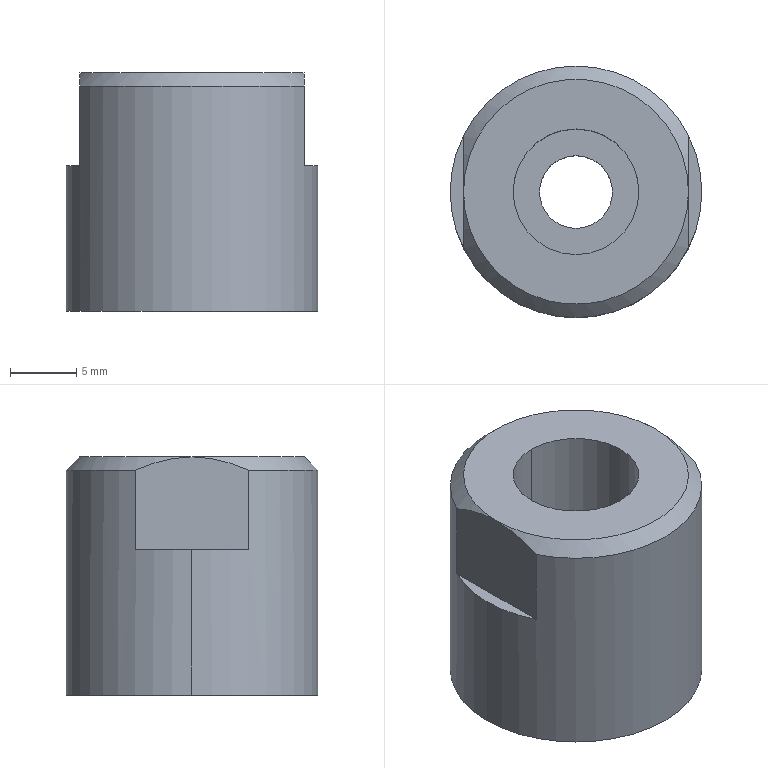Part | STEP file | J454-EBZ05-17-00-Part-1-16 | 1 solid | 15 faces | box 19 x 19 x 18 mm | volume 4103 mm3 | plane 7 | cylinder 6 | cone 2 | commonest cylinder face diameters 5.5 x2 9.5 x2 19 x2
STEP:
#1=CARTESIAN_POINT('',(0.,0.,0.));
#2=DIRECTION('',(0.,0.,1.));
#3=DIRECTION('',(1.,0.,0.));
#4=AXIS2_PLACEMENT_3D('',#1,#2,#3);
#5=CARTESIAN_POINT('',(0.,2.75,0.));
#6=VERTEX_POINT('',#5);
#7=CARTESIAN_POINT('',(0.,2.75,8.));
#8=VERTEX_POINT('',#7);
#9=CARTESIAN_POINT('',(0.,2.75,18.));
#10=DIRECTION('',(0.,0.,1.));
#11=VECTOR('',#10,1.);
#12=LINE('',#9,#11);
#13=CARTESIAN_POINT('',(0.,0.,18.));
#14=DIRECTION('',(0.,0.,1.));
#15=DIRECTION('',(0.,1.,0.));
#16=AXIS2_PLACEMENT_3D('',#13,#14,#15);
#17=CYLINDRICAL_SURFACE('',#16,2.75);
#18=CARTESIAN_POINT('',(6.283,0.));
#19=DIRECTION('',(0.,1.));
#20=VECTOR('',#19,1.);
#21=LINE('',#18,#20);
#22=(GEOMETRIC_REPRESENTATION_CONTEXT(2)PARAMETRIC_REPRESENTATION_CONTEXT()REPRESENTATION_CONTEXT('',''));
#23=DEFINITIONAL_REPRESENTATION('',(#21),#22);
#24=PCURVE('',#17,#23);
#25=CARTESIAN_POINT('',(0.,0.,18.));
#26=DIRECTION('',(0.,0.,1.));
#27=DIRECTION('',(0.,1.,0.));
#28=AXIS2_PLACEMENT_3D('',#25,#26,#27);
#29=CYLINDRICAL_SURFACE('',#28,2.75);
#30=CARTESIAN_POINT('',(0.,0.));
#31=DIRECTION('',(0.,1.));
#32=VECTOR('',#31,1.);
#33=LINE('',#30,#32);
#34=(GEOMETRIC_REPRESENTATION_CONTEXT(2)PARAMETRIC_REPRESENTATION_CONTEXT()REPRESENTATION_CONTEXT('',''));
#35=DEFINITIONAL_REPRESENTATION('',(#33),#34);
#36=PCURVE('',#29,#35);
#37=SURFACE_CURVE('',#12,(#24,#36),.PCURVE_S1.);
#38=EDGE_CURVE('',#6,#8,#37,.T.);
#39=ORIENTED_EDGE('',*,*,#38,.T.);
#40=CARTESIAN_POINT('',(0.,-2.75,8.));
#41=VERTEX_POINT('',#40);
#42=CARTESIAN_POINT('',(0.,0.,8.));
#43=DIRECTION('',(0.,0.,1.));
#44=DIRECTION('',(0.,1.,0.));
#45=AXIS2_PLACEMENT_3D('',#42,#43,#44);
#46=CIRCLE('',#45,2.75);
#47=CARTESIAN_POINT('',(0.,-10.));
#48=DIRECTION('',(1.,0.));
#49=VECTOR('',#48,1.);
#50=LINE('',#47,#49);
#51=(GEOMETRIC_REPRESENTATION_CONTEXT(2)PARAMETRIC_REPRESENTATION_CONTEXT()REPRESENTATION_CONTEXT('',''));
#52=DEFINITIONAL_REPRESENTATION('',(#50),#51);
#53=PCURVE('',#17,#52);
#54=CARTESIAN_POINT('',(0.,-4.75,8.));
#55=DIRECTION('',(0.,0.,-1.));
#56=DIRECTION('',(0.,-1.,0.));
#57=AXIS2_PLACEMENT_3D('',#54,#55,#56);
#58=PLANE('',#57);
#59=CARTESIAN_POINT('',(-7.5,0.));
#60=CARTESIAN_POINT('',(-7.5,4.763));
#61=CARTESIAN_POINT('',(-3.375,2.382));
#62=CARTESIAN_POINT('',(0.75,0.));
#63=CARTESIAN_POINT('',(-3.375,-2.382));
#64=CARTESIAN_POINT('',(-7.5,-4.763));
#65=CARTESIAN_POINT('',(-7.5,0.));
#66=(BOUNDED_CURVE()B_SPLINE_CURVE(2,(#59,#60,#61,#62,#63,#64,#65),.UNSPECIFIED.,.T.,.F.)B_SPLINE_CURVE_WITH_KNOTS((1,2,2,2,2,1),(-2.094,0.,2.094,4.189,6.283,8.378),.UNSPECIFIED.)CURVE()GEOMETRIC_REPRESENTATION_ITEM()RATIONAL_B_SPLINE_CURVE((1.,0.5,1.,0.5,1.,0.5,1.))REPRESENTATION_ITEM(''));
#67=(GEOMETRIC_REPRESENTATION_CONTEXT(2)PARAMETRIC_REPRESENTATION_CONTEXT()REPRESENTATION_CONTEXT('',''));
#68=DEFINITIONAL_REPRESENTATION('',(#66),#67);
#69=PCURVE('',#58,#68);
#70=SURFACE_CURVE('',#46,(#53,#69),.PCURVE_S1.);
#71=EDGE_CURVE('',#41,#8,#70,.T.);
#72=ORIENTED_EDGE('',*,*,#71,.F.);
#73=CARTESIAN_POINT('',(0.,-2.75,0.));
#74=VERTEX_POINT('',#73);
#75=CARTESIAN_POINT('',(0.,-2.75,18.));
#76=DIRECTION('',(0.,0.,1.));
#77=VECTOR('',#76,1.);
#78=LINE('',#75,#77);
#79=CARTESIAN_POINT('',(3.142,0.));
#80=DIRECTION('',(0.,1.));
#81=VECTOR('',#80,1.);
#82=LINE('',#79,#81);
#83=(GEOMETRIC_REPRESENTATION_CONTEXT(2)PARAMETRIC_REPRESENTATION_CONTEXT()REPRESENTATION_CONTEXT('',''));
#84=DEFINITIONAL_REPRESENTATION('',(#82),#83);
#85=PCURVE('',#17,#84);
#86=CARTESIAN_POINT('',(3.142,0.));
#87=DIRECTION('',(0.,1.));
#88=VECTOR('',#87,1.);
#89=LINE('',#86,#88);
#90=(GEOMETRIC_REPRESENTATION_CONTEXT(2)PARAMETRIC_REPRESENTATION_CONTEXT()REPRESENTATION_CONTEXT('',''));
#91=DEFINITIONAL_REPRESENTATION('',(#89),#90);
#92=PCURVE('',#29,#91);
#93=SURFACE_CURVE('',#78,(#85,#92),.PCURVE_S1.);
#94=EDGE_CURVE('',#74,#41,#93,.T.);
#95=ORIENTED_EDGE('',*,*,#94,.F.);
#96=CARTESIAN_POINT('',(0.,0.,0.));
#97=DIRECTION('',(0.,0.,1.));
#98=DIRECTION('',(0.,1.,0.));
#99=AXIS2_PLACEMENT_3D('',#96,#97,#98);
#100=CIRCLE('',#99,2.75);
#101=CARTESIAN_POINT('',(0.,-18.));
#102=DIRECTION('',(1.,0.));
#103=VECTOR('',#102,1.);
#104=LINE('',#101,#103);
#105=(GEOMETRIC_REPRESENTATION_CONTEXT(2)PARAMETRIC_REPRESENTATION_CONTEXT()REPRESENTATION_CONTEXT('',''));
#106=DEFINITIONAL_REPRESENTATION('',(#104),#105);
#107=PCURVE('',#17,#106);
#108=CARTESIAN_POINT('',(0.,0.,0.));
#109=DIRECTION('',(0.,0.,-1.));
#110=DIRECTION('',(-1.,0.,0.));
#111=AXIS2_PLACEMENT_3D('',#108,#109,#110);
#112=PLANE('',#111);
#113=CARTESIAN_POINT('',(0.,2.75));
#114=CARTESIAN_POINT('',(4.763,2.75));
#115=CARTESIAN_POINT('',(2.382,-1.375));
#116=CARTESIAN_POINT('',(0.,-5.5));
#117=CARTESIAN_POINT('',(-2.382,-1.375));
#118=CARTESIAN_POINT('',(-4.763,2.75));
#119=CARTESIAN_POINT('',(0.,2.75));
#120=(BOUNDED_CURVE()B_SPLINE_CURVE(2,(#113,#114,#115,#116,#117,#118,#119),.UNSPECIFIED.,.T.,.F.)B_SPLINE_CURVE_WITH_KNOTS((1,2,2,2,2,1),(-2.094,0.,2.094,4.189,6.283,8.378),.UNSPECIFIED.)CURVE()GEOMETRIC_REPRESENTATION_ITEM()RATIONAL_B_SPLINE_CURVE((1.,0.5,1.,0.5,1.,0.5,1.))REPRESENTATION_ITEM(''));
#121=(GEOMETRIC_REPRESENTATION_CONTEXT(2)PARAMETRIC_REPRESENTATION_CONTEXT()REPRESENTATION_CONTEXT('',''));
#122=DEFINITIONAL_REPRESENTATION('',(#120),#121);
#123=PCURVE('',#112,#122);
#124=SURFACE_CURVE('',#100,(#107,#123),.PCURVE_S1.);
#125=EDGE_CURVE('',#74,#6,#124,.T.);
#126=ORIENTED_EDGE('',*,*,#125,.T.);
#127=EDGE_LOOP('',(#39,#72,#95,#126));
#128=FACE_BOUND('',#127,.F.);
#129=ADVANCED_FACE('',(#128),#17,.F.);
#130=CARTESIAN_POINT('',(0.,4.75,8.));
#131=VERTEX_POINT('',#130);
#132=CARTESIAN_POINT('',(0.,4.75,18.));
#133=VERTEX_POINT('',#132);
#134=CARTESIAN_POINT('',(0.,4.75,18.));
#135=DIRECTION('',(0.,0.,1.));
#136=VECTOR('',#135,1.);
#137=LINE('',#134,#136);
#138=CARTESIAN_POINT('',(0.,0.,18.));
#139=DIRECTION('',(0.,0.,1.));
#140=DIRECTION('',(0.,1.,0.));
#141=AXIS2_PLACEMENT_3D('',#138,#139,#140);
#142=CYLINDRICAL_SURFACE('',#141,4.75);
#143=CARTESIAN_POINT('',(6.283,0.));
#144=DIRECTION('',(0.,1.));
#145=VECTOR('',#144,1.);
#146=LINE('',#143,#145);
#147=(GEOMETRIC_REPRESENTATION_CONTEXT(2)PARAMETRIC_REPRESENTATION_CONTEXT()REPRESENTATION_CONTEXT('',''));
#148=DEFINITIONAL_REPRESENTATION('',(#146),#147);
#149=PCURVE('',#142,#148);
#150=CARTESIAN_POINT('',(0.,0.,18.));
#151=DIRECTION('',(0.,0.,1.));
#152=DIRECTION('',(0.,1.,0.));
#153=AXIS2_PLACEMENT_3D('',#150,#151,#152);
#154=CYLINDRICAL_SURFACE('',#153,4.75);
#155=CARTESIAN_POINT('',(0.,0.));
#156=DIRECTION('',(0.,1.));
#157=VECTOR('',#156,1.);
#158=LINE('',#155,#157);
#159=(GEOMETRIC_REPRESENTATION_CONTEXT(2)PARAMETRIC_REPRESENTATION_CONTEXT()REPRESENTATION_CONTEXT('',''));
#160=DEFINITIONAL_REPRESENTATION('',(#158),#159);
#161=PCURVE('',#154,#160);
#162=SURFACE_CURVE('',#137,(#149,#161),.PCURVE_S1.);
#163=EDGE_CURVE('',#131,#133,#162,.T.);
#164=ORIENTED_EDGE('',*,*,#163,.T.);
#165=CARTESIAN_POINT('',(0.,-4.75,18.));
#166=VERTEX_POINT('',#165);
#167=CARTESIAN_POINT('',(0.,0.,18.));
#168=DIRECTION('',(0.,0.,1.));
#169=DIRECTION('',(0.,1.,0.));
#170=AXIS2_PLACEMENT_3D('',#167,#168,#169);
#171=CIRCLE('',#170,4.75);
#172=CARTESIAN_POINT('',(0.,0.));
#173=DIRECTION('',(1.,0.));
#174=VECTOR('',#173,1.);
#175=LINE('',#172,#174);
#176=(GEOMETRIC_REPRESENTATION_CONTEXT(2)PARAMETRIC_REPRESENTATION_CONTEXT()REPRESENTATION_CONTEXT('',''));
#177=DEFINITIONAL_REPRESENTATION('',(#175),#176);
#178=PCURVE('',#142,#177);
#179=CARTESIAN_POINT('',(0.,0.,18.));
#180=DIRECTION('',(0.,0.,1.));
#181=DIRECTION('',(1.,0.,0.));
#182=AXIS2_PLACEMENT_3D('',#179,#180,#181);
#183=PLANE('',#182);
#184=CARTESIAN_POINT('',(0.,0.));
#185=DIRECTION('',(0.,1.));
#186=AXIS2_PLACEMENT_2D('',#184,#185);
#187=CIRCLE('',#186,4.75);
#188=(GEOMETRIC_REPRESENTATION_CONTEXT(2)PARAMETRIC_REPRESENTATION_CONTEXT()REPRESENTATION_CONTEXT('',''));
#189=DEFINITIONAL_REPRESENTATION('',(#187),#188);
#190=PCURVE('',#183,#189);
#191=SURFACE_CURVE('',#171,(#178,#190),.PCURVE_S1.);
#192=EDGE_CURVE('',#166,#133,#191,.T.);
#193=ORIENTED_EDGE('',*,*,#192,.F.);
#194=CARTESIAN_POINT('',(0.,-4.75,8.));
#195=VERTEX_POINT('',#194);
#196=CARTESIAN_POINT('',(0.,-4.75,18.));
#197=DIRECTION('',(0.,0.,1.));
#198=VECTOR('',#197,1.);
#199=LINE('',#196,#198);
#200=CARTESIAN_POINT('',(3.142,0.));
#201=DIRECTION('',(0.,1.));
#202=VECTOR('',#201,1.);
#203=LINE('',#200,#202);
#204=(GEOMETRIC_REPRESENTATION_CONTEXT(2)PARAMETRIC_REPRESENTATION_CONTEXT()REPRESENTATION_CONTEXT('',''));
#205=DEFINITIONAL_REPRESENTATION('',(#203),#204);
#206=PCURVE('',#142,#205);
#207=CARTESIAN_POINT('',(3.142,0.));
#208=DIRECTION('',(0.,1.));
#209=VECTOR('',#208,1.);
#210=LINE('',#207,#209);
#211=(GEOMETRIC_REPRESENTATION_CONTEXT(2)PARAMETRIC_REPRESENTATION_CONTEXT()REPRESENTATION_CONTEXT('',''));
#212=DEFINITIONAL_REPRESENTATION('',(#210),#211);
#213=PCURVE('',#154,#212);
#214=SURFACE_CURVE('',#199,(#206,#213),.PCURVE_S1.);
#215=EDGE_CURVE('',#195,#166,#214,.T.);
#216=ORIENTED_EDGE('',*,*,#215,.F.);
#217=CARTESIAN_POINT('',(0.,0.,8.));
#218=DIRECTION('',(0.,0.,1.));
#219=DIRECTION('',(0.,1.,0.));
#220=AXIS2_PLACEMENT_3D('',#217,#218,#219);
#221=CIRCLE('',#220,4.75);
#222=CARTESIAN_POINT('',(0.,-10.));
#223=DIRECTION('',(1.,0.));
#224=VECTOR('',#223,1.);
#225=LINE('',#222,#224);
#226=(GEOMETRIC_REPRESENTATION_CONTEXT(2)PARAMETRIC_REPRESENTATION_CONTEXT()REPRESENTATION_CONTEXT('',''));
#227=DEFINITIONAL_REPRESENTATION('',(#225),#226);
#228=PCURVE('',#142,#227);
#229=CARTESIAN_POINT('',(-9.5,0.));
#230=CARTESIAN_POINT('',(-9.5,8.227));
#231=CARTESIAN_POINT('',(-2.375,4.114));
#232=CARTESIAN_POINT('',(4.75,0.));
#233=CARTESIAN_POINT('',(-2.375,-4.114));
#234=CARTESIAN_POINT('',(-9.5,-8.227));
#235=CARTESIAN_POINT('',(-9.5,0.));
#236=(BOUNDED_CURVE()B_SPLINE_CURVE(2,(#229,#230,#231,#232,#233,#234,#235),.UNSPECIFIED.,.T.,.F.)B_SPLINE_CURVE_WITH_KNOTS((1,2,2,2,2,1),(-2.094,0.,2.094,4.189,6.283,8.378),.UNSPECIFIED.)CURVE()GEOMETRIC_REPRESENTATION_ITEM()RATIONAL_B_SPLINE_CURVE((1.,0.5,1.,0.5,1.,0.5,1.))REPRESENTATION_ITEM(''));
#237=(GEOMETRIC_REPRESENTATION_CONTEXT(2)PARAMETRIC_REPRESENTATION_CONTEXT()REPRESENTATION_CONTEXT('',''));
#238=DEFINITIONAL_REPRESENTATION('',(#236),#237);
#239=PCURVE('',#58,#238);
#240=SURFACE_CURVE('',#221,(#228,#239),.PCURVE_S1.);
#241=EDGE_CURVE('',#195,#131,#240,.T.);
#242=ORIENTED_EDGE('',*,*,#241,.T.);
#243=EDGE_LOOP('',(#164,#193,#216,#242));
#244=FACE_BOUND('',#243,.F.);
#245=ADVANCED_FACE('',(#244),#142,.F.);
#246=CARTESIAN_POINT('',(9.5,0.,0.));
#247=VERTEX_POINT('',#246);
#248=CARTESIAN_POINT('',(-9.5,0.,0.));
#249=VERTEX_POINT('',#248);
#250=CARTESIAN_POINT('',(0.,0.,0.));
#251=DIRECTION('',(0.,0.,1.));
#252=DIRECTION('',(1.,0.,0.));
#253=AXIS2_PLACEMENT_3D('',#250,#251,#252);
#254=CIRCLE('',#253,9.5);
#255=CARTESIAN_POINT('',(0.,0.,0.));
#256=DIRECTION('',(0.,0.,1.));
#257=DIRECTION('',(1.,0.,0.));
#258=AXIS2_PLACEMENT_3D('',#255,#256,#257);
#259=CYLINDRICAL_SURFACE('',#258,9.5);
#260=CARTESIAN_POINT('',(0.,0.));
#261=DIRECTION('',(1.,0.));
#262=VECTOR('',#261,1.);
#263=LINE('',#260,#262);
#264=(GEOMETRIC_REPRESENTATION_CONTEXT(2)PARAMETRIC_REPRESENTATION_CONTEXT()REPRESENTATION_CONTEXT('',''));
#265=DEFINITIONAL_REPRESENTATION('',(#263),#264);
#266=PCURVE('',#259,#265);
#267=CARTESIAN_POINT('',(-9.5,0.));
#268=CARTESIAN_POINT('',(-9.5,16.454));
#269=CARTESIAN_POINT('',(4.75,8.227));
#270=CARTESIAN_POINT('',(19.,0.));
#271=CARTESIAN_POINT('',(4.75,-8.227));
#272=CARTESIAN_POINT('',(-9.5,-16.454));
#273=CARTESIAN_POINT('',(-9.5,0.));
#274=(BOUNDED_CURVE()B_SPLINE_CURVE(2,(#267,#268,#269,#270,#271,#272,#273),.UNSPECIFIED.,.T.,.F.)B_SPLINE_CURVE_WITH_KNOTS((1,2,2,2,2,1),(-2.094,0.,2.094,4.189,6.283,8.378),.UNSPECIFIED.)CURVE()GEOMETRIC_REPRESENTATION_ITEM()RATIONAL_B_SPLINE_CURVE((1.,0.5,1.,0.5,1.,0.5,1.))REPRESENTATION_ITEM(''));
#275=(GEOMETRIC_REPRESENTATION_CONTEXT(2)PARAMETRIC_REPRESENTATION_CONTEXT()REPRESENTATION_CONTEXT('',''));
#276=DEFINITIONAL_REPRESENTATION('',(#274),#275);
#277=PCURVE('',#112,#276);
#278=SURFACE_CURVE('',#254,(#266,#277),.PCURVE_S1.);
#279=EDGE_CURVE('',#247,#249,#278,.T.);
#280=ORIENTED_EDGE('',*,*,#279,.T.);
#281=CARTESIAN_POINT('',(-9.5,0.,11.));
#282=VERTEX_POINT('',#281);
#283=CARTESIAN_POINT('',(-9.5,0.,0.));
#284=DIRECTION('',(0.,0.,1.));
#285=VECTOR('',#284,1.);
#286=LINE('',#283,#285);
#287=CARTESIAN_POINT('',(3.142,0.));
#288=DIRECTION('',(0.,1.));
#289=VECTOR('',#288,1.);
#290=LINE('',#287,#289);
#291=(GEOMETRIC_REPRESENTATION_CONTEXT(2)PARAMETRIC_REPRESENTATION_CONTEXT()REPRESENTATION_CONTEXT('',''));
#292=DEFINITIONAL_REPRESENTATION('',(#290),#291);
#293=PCURVE('',#259,#292);
#294=CARTESIAN_POINT('',(0.,0.,0.));
#295=DIRECTION('',(0.,0.,1.));
#296=DIRECTION('',(1.,0.,0.));
#297=AXIS2_PLACEMENT_3D('',#294,#295,#296);
#298=CYLINDRICAL_SURFACE('',#297,9.5);
#299=CARTESIAN_POINT('',(3.142,0.));
#300=DIRECTION('',(0.,1.));
#301=VECTOR('',#300,1.);
#302=LINE('',#299,#301);
#303=(GEOMETRIC_REPRESENTATION_CONTEXT(2)PARAMETRIC_REPRESENTATION_CONTEXT()REPRESENTATION_CONTEXT('',''));
#304=DEFINITIONAL_REPRESENTATION('',(#302),#303);
#305=PCURVE('',#298,#304);
#306=SURFACE_CURVE('',#286,(#293,#305),.PCURVE_S1.);
#307=EDGE_CURVE('',#249,#282,#306,.T.);
#308=ORIENTED_EDGE('',*,*,#307,.T.);
#309=CARTESIAN_POINT('',(-8.5,4.243,11.));
#310=VERTEX_POINT('',#309);
#311=CARTESIAN_POINT('',(0.,0.,11.));
#312=DIRECTION('',(0.,0.,1.));
#313=DIRECTION('',(-1.,0.,0.));
#314=AXIS2_PLACEMENT_3D('',#311,#312,#313);
#315=CIRCLE('',#314,9.5);
#316=CARTESIAN_POINT('',(-3.142,11.));
#317=DIRECTION('',(1.,0.));
#318=VECTOR('',#317,1.);
#319=LINE('',#316,#318);
#320=(GEOMETRIC_REPRESENTATION_CONTEXT(2)PARAMETRIC_REPRESENTATION_CONTEXT()REPRESENTATION_CONTEXT('',''));
#321=DEFINITIONAL_REPRESENTATION('',(#319),#320);
#322=PCURVE('',#259,#321);
#323=CARTESIAN_POINT('',(-19.25,-7.5,11.));
#324=DIRECTION('',(0.,0.,-1.));
#325=DIRECTION('',(0.,-1.,0.));
#326=AXIS2_PLACEMENT_3D('',#323,#324,#325);
#327=PLANE('',#326);
#328=CARTESIAN_POINT('',(-7.5,-9.75));
#329=CARTESIAN_POINT('',(8.954,-9.75));
#330=CARTESIAN_POINT('',(0.7272,-24.));
#331=CARTESIAN_POINT('',(-7.5,-38.25));
#332=CARTESIAN_POINT('',(-15.727,-24.));
#333=CARTESIAN_POINT('',(-23.954,-9.75));
#334=CARTESIAN_POINT('',(-7.5,-9.75));
#335=(BOUNDED_CURVE()B_SPLINE_CURVE(2,(#328,#329,#330,#331,#332,#333,#334),.UNSPECIFIED.,.T.,.F.)B_SPLINE_CURVE_WITH_KNOTS((1,2,2,2,2,1),(-2.094,0.,2.094,4.189,6.283,8.378),.UNSPECIFIED.)CURVE()GEOMETRIC_REPRESENTATION_ITEM()RATIONAL_B_SPLINE_CURVE((1.,0.5,1.,0.5,1.,0.5,1.))REPRESENTATION_ITEM(''));
#336=(GEOMETRIC_REPRESENTATION_CONTEXT(2)PARAMETRIC_REPRESENTATION_CONTEXT()REPRESENTATION_CONTEXT('',''));
#337=DEFINITIONAL_REPRESENTATION('',(#335),#336);
#338=PCURVE('',#327,#337);
#339=SURFACE_CURVE('',#315,(#322,#338),.PCURVE_S1.);
#340=EDGE_CURVE('',#310,#282,#339,.T.);
#341=ORIENTED_EDGE('',*,*,#340,.F.);
#342=CARTESIAN_POINT('',(-8.5,4.243,17.));
#343=VERTEX_POINT('',#342);
#344=CARTESIAN_POINT('',(-8.5,4.243,0.));
#345=DIRECTION('',(0.,0.,-1.));
#346=VECTOR('',#345,1.);
#347=LINE('',#344,#346);
#348=CARTESIAN_POINT('',(2.679,0.));
#349=DIRECTION('',(0.,-1.));
#350=VECTOR('',#349,1.);
#351=LINE('',#348,#350);
#352=(GEOMETRIC_REPRESENTATION_CONTEXT(2)PARAMETRIC_REPRESENTATION_CONTEXT()REPRESENTATION_CONTEXT('',''));
#353=DEFINITIONAL_REPRESENTATION('',(#351),#352);
#354=PCURVE('',#259,#353);
#355=CARTESIAN_POINT('',(-8.5,-7.5,14.5));
#356=DIRECTION('',(1.,0.,0.));
#357=DIRECTION('',(0.,1.,0.));
#358=AXIS2_PLACEMENT_3D('',#355,#356,#357);
#359=PLANE('',#358);
#360=CARTESIAN_POINT('',(11.743,-14.5));
#361=DIRECTION('',(0.,-1.));
#362=VECTOR('',#361,1.);
#363=LINE('',#360,#362);
#364=(GEOMETRIC_REPRESENTATION_CONTEXT(2)PARAMETRIC_REPRESENTATION_CONTEXT()REPRESENTATION_CONTEXT('',''));
#365=DEFINITIONAL_REPRESENTATION('',(#363),#364);
#366=PCURVE('',#359,#365);
#367=SURFACE_CURVE('',#347,(#354,#366),.PCURVE_S1.);
#368=EDGE_CURVE('',#343,#310,#367,.T.);
#369=ORIENTED_EDGE('',*,*,#368,.F.);
#370=CARTESIAN_POINT('',(8.5,4.243,17.));
#371=VERTEX_POINT('',#370);
#372=CARTESIAN_POINT('',(0.,0.,17.));
#373=DIRECTION('',(0.,0.,-1.));
#374=DIRECTION('',(1.,0.,0.));
#375=AXIS2_PLACEMENT_3D('',#372,#373,#374);
#376=CIRCLE('',#375,9.5);
#377=CARTESIAN_POINT('',(6.283,17.));
#378=DIRECTION('',(-1.,0.));
#379=VECTOR('',#378,1.);
#380=LINE('',#377,#379);
#381=(GEOMETRIC_REPRESENTATION_CONTEXT(2)PARAMETRIC_REPRESENTATION_CONTEXT()REPRESENTATION_CONTEXT('',''));
#382=DEFINITIONAL_REPRESENTATION('',(#380),#381);
#383=PCURVE('',#259,#382);
#384=CARTESIAN_POINT('',(0.,0.,17.));
#385=DIRECTION('',(0.,0.,-1.));
#386=DIRECTION('',(-1.,0.,0.));
#387=AXIS2_PLACEMENT_3D('',#384,#385,#386);
#388=CONICAL_SURFACE('',#387,9.5,0.7854);
#389=CARTESIAN_POINT('',(-3.142,0.));
#390=DIRECTION('',(1.,0.));
#391=VECTOR('',#390,1.);
#392=LINE('',#389,#391);
#393=(GEOMETRIC_REPRESENTATION_CONTEXT(2)PARAMETRIC_REPRESENTATION_CONTEXT()REPRESENTATION_CONTEXT('',''));
#394=DEFINITIONAL_REPRESENTATION('',(#392),#393);
#395=PCURVE('',#388,#394);
#396=SURFACE_CURVE('',#376,(#383,#395),.PCURVE_S1.);
#397=EDGE_CURVE('',#343,#371,#396,.T.);
#398=ORIENTED_EDGE('',*,*,#397,.T.);
#399=CARTESIAN_POINT('',(8.5,4.243,11.));
#400=VERTEX_POINT('',#399);
#401=CARTESIAN_POINT('',(8.5,4.243,0.));
#402=DIRECTION('',(0.,0.,1.));
#403=VECTOR('',#402,1.);
#404=LINE('',#401,#403);
#405=CARTESIAN_POINT('',(0.463,0.));
#406=DIRECTION('',(0.,1.));
#407=VECTOR('',#406,1.);
#408=LINE('',#405,#407);
#409=(GEOMETRIC_REPRESENTATION_CONTEXT(2)PARAMETRIC_REPRESENTATION_CONTEXT()REPRESENTATION_CONTEXT('',''));
#410=DEFINITIONAL_REPRESENTATION('',(#408),#409);
#411=PCURVE('',#259,#410);
#412=CARTESIAN_POINT('',(8.5,7.5,14.5));
#413=DIRECTION('',(-1.,0.,0.));
#414=DIRECTION('',(0.,-1.,0.));
#415=AXIS2_PLACEMENT_3D('',#412,#413,#414);
#416=PLANE('',#415);
#417=CARTESIAN_POINT('',(3.257,-14.5));
#418=DIRECTION('',(0.,1.));
#419=VECTOR('',#418,1.);
#420=LINE('',#417,#419);
#421=(GEOMETRIC_REPRESENTATION_CONTEXT(2)PARAMETRIC_REPRESENTATION_CONTEXT()REPRESENTATION_CONTEXT('',''));
#422=DEFINITIONAL_REPRESENTATION('',(#420),#421);
#423=PCURVE('',#416,#422);
#424=SURFACE_CURVE('',#404,(#411,#423),.PCURVE_S1.);
#425=EDGE_CURVE('',#400,#371,#424,.T.);
#426=ORIENTED_EDGE('',*,*,#425,.F.);
#427=CARTESIAN_POINT('',(9.5,0.,11.));
#428=VERTEX_POINT('',#427);
#429=CARTESIAN_POINT('',(0.,0.,11.));
#430=DIRECTION('',(0.,0.,1.));
#431=DIRECTION('',(-1.,0.,0.));
#432=AXIS2_PLACEMENT_3D('',#429,#430,#431);
#433=CIRCLE('',#432,9.5);
#434=CARTESIAN_POINT('',(-3.142,11.));
#435=DIRECTION('',(1.,0.));
#436=VECTOR('',#435,1.);
#437=LINE('',#434,#436);
#438=(GEOMETRIC_REPRESENTATION_CONTEXT(2)PARAMETRIC_REPRESENTATION_CONTEXT()REPRESENTATION_CONTEXT('',''));
#439=DEFINITIONAL_REPRESENTATION('',(#437),#438);
#440=PCURVE('',#259,#439);
#441=CARTESIAN_POINT('',(19.25,7.5,11.));
#442=DIRECTION('',(0.,0.,-1.));
#443=DIRECTION('',(0.,1.,0.));
#444=AXIS2_PLACEMENT_3D('',#441,#442,#443);
#445=PLANE('',#444);
#446=CARTESIAN_POINT('',(-7.5,-28.75));
#447=CARTESIAN_POINT('',(-23.954,-28.75));
#448=CARTESIAN_POINT('',(-15.727,-14.5));
#449=CARTESIAN_POINT('',(-7.5,-0.25));
#450=CARTESIAN_POINT('',(0.7272,-14.5));
#451=CARTESIAN_POINT('',(8.954,-28.75));
#452=CARTESIAN_POINT('',(-7.5,-28.75));
#453=(BOUNDED_CURVE()B_SPLINE_CURVE(2,(#446,#447,#448,#449,#450,#451,#452),.UNSPECIFIED.,.T.,.F.)B_SPLINE_CURVE_WITH_KNOTS((1,2,2,2,2,1),(-2.094,0.,2.094,4.189,6.283,8.378),.UNSPECIFIED.)CURVE()GEOMETRIC_REPRESENTATION_ITEM()RATIONAL_B_SPLINE_CURVE((1.,0.5,1.,0.5,1.,0.5,1.))REPRESENTATION_ITEM(''));
#454=(GEOMETRIC_REPRESENTATION_CONTEXT(2)PARAMETRIC_REPRESENTATION_CONTEXT()REPRESENTATION_CONTEXT('',''));
#455=DEFINITIONAL_REPRESENTATION('',(#453),#454);
#456=PCURVE('',#445,#455);
#457=SURFACE_CURVE('',#433,(#440,#456),.PCURVE_S1.);
#458=EDGE_CURVE('',#428,#400,#457,.T.);
#459=ORIENTED_EDGE('',*,*,#458,.F.);
#460=CARTESIAN_POINT('',(9.5,0.,0.));
#461=DIRECTION('',(0.,0.,1.));
#462=VECTOR('',#461,1.);
#463=LINE('',#460,#462);
#464=CARTESIAN_POINT('',(0.,0.));
#465=DIRECTION('',(0.,1.));
#466=VECTOR('',#465,1.);
#467=LINE('',#464,#466);
#468=(GEOMETRIC_REPRESENTATION_CONTEXT(2)PARAMETRIC_REPRESENTATION_CONTEXT()REPRESENTATION_CONTEXT('',''));
#469=DEFINITIONAL_REPRESENTATION('',(#467),#468);
#470=PCURVE('',#259,#469);
#471=CARTESIAN_POINT('',(6.283,0.));
#472=DIRECTION('',(0.,1.));
#473=VECTOR('',#472,1.);
#474=LINE('',#471,#473);
#475=(GEOMETRIC_REPRESENTATION_CONTEXT(2)PARAMETRIC_REPRESENTATION_CONTEXT()REPRESENTATION_CONTEXT('',''));
#476=DEFINITIONAL_REPRESENTATION('',(#474),#475);
#477=PCURVE('',#298,#476);
#478=SURFACE_CURVE('',#463,(#470,#477),.PCURVE_S1.);
#479=EDGE_CURVE('',#247,#428,#478,.T.);
#480=ORIENTED_EDGE('',*,*,#479,.F.);
#481=EDGE_LOOP('',(#280,#308,#341,#369,#398,#426,#459,#480));
#482=FACE_BOUND('',#481,.T.);
#483=ADVANCED_FACE('',(#482),#259,.T.);
#484=CARTESIAN_POINT('',(8.5,0.,18.));
#485=VERTEX_POINT('',#484);
#486=CARTESIAN_POINT('',(8.5,4.243,17.));
#487=CARTESIAN_POINT('',(8.5,3.909,17.149));
#488=CARTESIAN_POINT('',(8.5,3.57,17.287));
#489=CARTESIAN_POINT('',(8.5,2.877,17.532));
#490=CARTESIAN_POINT('',(8.5,2.524,17.64));
#491=CARTESIAN_POINT('',(8.5,1.459,17.903));
#492=CARTESIAN_POINT('',(8.5,0.737,18.));
#493=CARTESIAN_POINT('',(8.5,0.,18.));
#494=B_SPLINE_CURVE_WITH_KNOTS('',3,(#486,#487,#488,#489,#490,#491,#492,#493),.UNSPECIFIED.,.F.,.F.,(4,2,2,4),(0.02347,0.02457,0.02567,0.02786),.UNSPECIFIED.);
#495=CARTESIAN_POINT('',(2.679,0.));
#496=CARTESIAN_POINT('',(2.684,-0.0271));
#497=CARTESIAN_POINT('',(2.696,-0.08054));
#498=CARTESIAN_POINT('',(2.714,-0.1583));
#499=CARTESIAN_POINT('',(2.732,-0.2335));
#500=CARTESIAN_POINT('',(2.75,-0.3061));
#501=CARTESIAN_POINT('',(2.769,-0.376));
#502=CARTESIAN_POINT('',(2.789,-0.443));
#503=CARTESIAN_POINT('',(2.809,-0.5069));
#504=CARTESIAN_POINT('',(2.829,-0.5676));
#505=CARTESIAN_POINT('',(2.85,-0.6249));
#506=CARTESIAN_POINT('',(2.87,-0.6785));
#507=CARTESIAN_POINT('',(2.892,-0.7283));
#508=CARTESIAN_POINT('',(2.913,-0.7742));
#509=CARTESIAN_POINT('',(2.935,-0.8162));
#510=CARTESIAN_POINT('',(2.957,-0.8541));
#511=CARTESIAN_POINT('',(2.98,-0.8878));
#512=CARTESIAN_POINT('',(3.002,-0.9173));
#513=CARTESIAN_POINT('',(3.025,-0.9425));
#514=CARTESIAN_POINT('',(3.048,-0.9633));
#515=CARTESIAN_POINT('',(3.071,-0.9796));
#516=CARTESIAN_POINT('',(3.094,-0.9913));
#517=CARTESIAN_POINT('',(3.118,-0.9984));
#518=CARTESIAN_POINT('',(3.134,-1.));
#519=CARTESIAN_POINT('',(3.142,-1.));
#520=B_SPLINE_CURVE_WITH_KNOTS('',3,(#495,#496,#497,#498,#499,#500,#501,#502,#503,#504,#505,#506,#507,#508,#509,#510,#511,#512,#513,#514,#515,#516,#517,#518,#519),.UNSPECIFIED.,.F.,.F.,(4,1,1,1,1,1,1,1,1,1,1,1,1,1,1,1,1,1,1,1,1,1,4),(0.02347,0.02367,0.02387,0.02407,0.02427,0.02447,0.02467,0.02487,0.02507,0.02527,0.02547,0.02567,0.02587,0.02607,0.02627,0.02647,0.02667,0.02687,0.02707,0.02727,0.02747,0.02766,0.02786),.QUASI_UNIFORM_KNOTS.);
#521=(GEOMETRIC_REPRESENTATION_CONTEXT(2)PARAMETRIC_REPRESENTATION_CONTEXT()REPRESENTATION_CONTEXT('',''));
#522=DEFINITIONAL_REPRESENTATION('',(#520),#521);
#523=PCURVE('',#388,#522);
#524=CARTESIAN_POINT('',(3.257,2.5));
#525=CARTESIAN_POINT('',(3.591,2.649));
#526=CARTESIAN_POINT('',(3.93,2.787));
#527=CARTESIAN_POINT('',(4.623,3.032));
#528=CARTESIAN_POINT('',(4.976,3.14));
#529=CARTESIAN_POINT('',(6.041,3.403));
#530=CARTESIAN_POINT('',(6.763,3.5));
#531=CARTESIAN_POINT('',(7.5,3.5));
#532=B_SPLINE_CURVE_WITH_KNOTS('',3,(#524,#525,#526,#527,#528,#529,#530,#531),.UNSPECIFIED.,.F.,.F.,(4,2,2,4),(0.02347,0.02457,0.02567,0.02786),.UNSPECIFIED.);
#533=(GEOMETRIC_REPRESENTATION_CONTEXT(2)PARAMETRIC_REPRESENTATION_CONTEXT()REPRESENTATION_CONTEXT('',''));
#534=DEFINITIONAL_REPRESENTATION('',(#532),#533);
#535=PCURVE('',#416,#534);
#536=SURFACE_CURVE('',#494,(#523,#535),.PCURVE_S1.);
#537=EDGE_CURVE('',#371,#485,#536,.T.);
#538=ORIENTED_EDGE('',*,*,#537,.F.);
#539=ORIENTED_EDGE('',*,*,#397,.F.);
#540=CARTESIAN_POINT('',(-8.5,0.,18.));
#541=VERTEX_POINT('',#540);
#542=CARTESIAN_POINT('',(-8.5,0.,18.));
#543=CARTESIAN_POINT('',(-8.5,0.3684,18.));
#544=CARTESIAN_POINT('',(-8.5,0.7366,17.976));
#545=CARTESIAN_POINT('',(-8.5,1.461,17.883));
#546=CARTESIAN_POINT('',(-8.5,1.818,17.814));
#547=CARTESIAN_POINT('',(-8.5,2.881,17.551));
#548=CARTESIAN_POINT('',(-8.5,3.578,17.297));
#549=CARTESIAN_POINT('',(-8.5,4.243,17.));
#550=B_SPLINE_CURVE_WITH_KNOTS('',3,(#542,#543,#544,#545,#546,#547,#548,#549),.UNSPECIFIED.,.F.,.F.,(4,2,2,4),(0.02786,0.02896,0.03006,0.03225),.UNSPECIFIED.);
#551=CARTESIAN_POINT('',(0.,-1.));
#552=CARTESIAN_POINT('',(0.00788,-1.));
#553=CARTESIAN_POINT('',(0.02364,-0.9984));
#554=CARTESIAN_POINT('',(0.04722,-0.9913));
#555=CARTESIAN_POINT('',(0.0707,-0.9795));
#556=CARTESIAN_POINT('',(0.09401,-0.9631));
#557=CARTESIAN_POINT('',(0.1171,-0.9421));
#558=CARTESIAN_POINT('',(0.14,-0.9168));
#559=CARTESIAN_POINT('',(0.1626,-0.8872));
#560=CARTESIAN_POINT('',(0.1849,-0.8533));
#561=CARTESIAN_POINT('',(0.207,-0.8153));
#562=CARTESIAN_POINT('',(0.2288,-0.7733));
#563=CARTESIAN_POINT('',(0.2503,-0.7274));
#564=CARTESIAN_POINT('',(0.2715,-0.6776));
#565=CARTESIAN_POINT('',(0.2923,-0.6241));
#566=CARTESIAN_POINT('',(0.3129,-0.567));
#567=CARTESIAN_POINT('',(0.333,-0.5065));
#568=CARTESIAN_POINT('',(0.3528,-0.4427));
#569=CARTESIAN_POINT('',(0.3722,-0.3757));
#570=CARTESIAN_POINT('',(0.3912,-0.3059));
#571=CARTESIAN_POINT('',(0.4098,-0.2332));
#572=CARTESIAN_POINT('',(0.428,-0.158));
#573=CARTESIAN_POINT('',(0.4457,-0.08029));
#574=CARTESIAN_POINT('',(0.4573,-0.02699));
#575=CARTESIAN_POINT('',(0.463,0.));
#576=B_SPLINE_CURVE_WITH_KNOTS('',3,(#551,#552,#553,#554,#555,#556,#557,#558,#559,#560,#561,#562,#563,#564,#565,#566,#567,#568,#569,#570,#571,#572,#573,#574,#575),.UNSPECIFIED.,.F.,.F.,(4,1,1,1,1,1,1,1,1,1,1,1,1,1,1,1,1,1,1,1,1,1,4),(0.02786,0.02806,0.02826,0.02846,0.02866,0.02886,0.02906,0.02926,0.02946,0.02966,0.02986,0.03006,0.03026,0.03046,0.03066,0.03086,0.03106,0.03126,0.03145,0.03165,0.03185,0.03205,0.03225),.QUASI_UNIFORM_KNOTS.);
#577=(GEOMETRIC_REPRESENTATION_CONTEXT(2)PARAMETRIC_REPRESENTATION_CONTEXT()REPRESENTATION_CONTEXT('',''));
#578=DEFINITIONAL_REPRESENTATION('',(#576),#577);
#579=PCURVE('',#388,#578);
#580=CARTESIAN_POINT('',(7.5,3.5));
#581=CARTESIAN_POINT('',(7.868,3.5));
#582=CARTESIAN_POINT('',(8.237,3.476));
#583=CARTESIAN_POINT('',(8.961,3.383));
#584=CARTESIAN_POINT('',(9.318,3.314));
#585=CARTESIAN_POINT('',(10.381,3.051));
#586=CARTESIAN_POINT('',(11.078,2.797));
#587=CARTESIAN_POINT('',(11.743,2.5));
#588=B_SPLINE_CURVE_WITH_KNOTS('',3,(#580,#581,#582,#583,#584,#585,#586,#587),.UNSPECIFIED.,.F.,.F.,(4,2,2,4),(0.02786,0.02896,0.03006,0.03225),.UNSPECIFIED.);
#589=(GEOMETRIC_REPRESENTATION_CONTEXT(2)PARAMETRIC_REPRESENTATION_CONTEXT()REPRESENTATION_CONTEXT('',''));
#590=DEFINITIONAL_REPRESENTATION('',(#588),#589);
#591=PCURVE('',#359,#590);
#592=SURFACE_CURVE('',#550,(#579,#591),.PCURVE_S1.);
#593=EDGE_CURVE('',#541,#343,#592,.T.);
#594=ORIENTED_EDGE('',*,*,#593,.F.);
#595=CARTESIAN_POINT('',(0.,0.,18.));
#596=DIRECTION('',(0.,0.,1.));
#597=DIRECTION('',(1.,0.,0.));
#598=AXIS2_PLACEMENT_3D('',#595,#596,#597);
#599=CIRCLE('',#598,8.5);
#600=CARTESIAN_POINT('',(3.142,-1.));
#601=DIRECTION('',(-1.,0.));
#602=VECTOR('',#601,1.);
#603=LINE('',#600,#602);
#604=(GEOMETRIC_REPRESENTATION_CONTEXT(2)PARAMETRIC_REPRESENTATION_CONTEXT()REPRESENTATION_CONTEXT('',''));
#605=DEFINITIONAL_REPRESENTATION('',(#603),#604);
#606=PCURVE('',#388,#605);
#607=CARTESIAN_POINT('',(0.,0.));
#608=DIRECTION('',(1.,0.));
#609=AXIS2_PLACEMENT_2D('',#607,#608);
#610=CIRCLE('',#609,8.5);
#611=(GEOMETRIC_REPRESENTATION_CONTEXT(2)PARAMETRIC_REPRESENTATION_CONTEXT()REPRESENTATION_CONTEXT('',''));
#612=DEFINITIONAL_REPRESENTATION('',(#610),#611);
#613=PCURVE('',#183,#612);
#614=SURFACE_CURVE('',#599,(#606,#613),.PCURVE_S1.);
#615=EDGE_CURVE('',#485,#541,#614,.T.);
#616=ORIENTED_EDGE('',*,*,#615,.F.);
#617=EDGE_LOOP('',(#538,#539,#594,#616));
#618=FACE_BOUND('',#617,.T.);
#619=ADVANCED_FACE('',(#618),#388,.T.);
#620=CARTESIAN_POINT('',(0.,0.,18.));
#621=DIRECTION('',(0.,0.,1.));
#622=DIRECTION('',(0.,1.,0.));
#623=AXIS2_PLACEMENT_3D('',#620,#621,#622);
#624=CIRCLE('',#623,4.75);
#625=CARTESIAN_POINT('',(0.,0.));
#626=DIRECTION('',(0.,1.));
#627=AXIS2_PLACEMENT_2D('',#625,#626);
#628=CIRCLE('',#627,4.75);
#629=(GEOMETRIC_REPRESENTATION_CONTEXT(2)PARAMETRIC_REPRESENTATION_CONTEXT()REPRESENTATION_CONTEXT('',''));
#630=DEFINITIONAL_REPRESENTATION('',(#628),#629);
#631=PCURVE('',#183,#630);
#632=CARTESIAN_POINT('',(0.,0.));
#633=DIRECTION('',(1.,0.));
#634=VECTOR('',#633,1.);
#635=LINE('',#632,#634);
#636=(GEOMETRIC_REPRESENTATION_CONTEXT(2)PARAMETRIC_REPRESENTATION_CONTEXT()REPRESENTATION_CONTEXT('',''));
#637=DEFINITIONAL_REPRESENTATION('',(#635),#636);
#638=PCURVE('',#154,#637);
#639=SURFACE_CURVE('',#624,(#631,#638),.PCURVE_S1.);
#640=EDGE_CURVE('',#133,#166,#639,.T.);
#641=ORIENTED_EDGE('',*,*,#640,.F.);
#642=ORIENTED_EDGE('',*,*,#192,.F.);
#643=EDGE_LOOP('',(#641,#642));
#644=FACE_BOUND('',#643,.T.);
#645=CARTESIAN_POINT('',(0.,0.,18.));
#646=DIRECTION('',(0.,0.,1.));
#647=DIRECTION('',(1.,0.,0.));
#648=AXIS2_PLACEMENT_3D('',#645,#646,#647);
#649=CIRCLE('',#648,8.5);
#650=CARTESIAN_POINT('',(0.,0.));
#651=DIRECTION('',(1.,0.));
#652=AXIS2_PLACEMENT_2D('',#650,#651);
#653=CIRCLE('',#652,8.5);
#654=(GEOMETRIC_REPRESENTATION_CONTEXT(2)PARAMETRIC_REPRESENTATION_CONTEXT()REPRESENTATION_CONTEXT('',''));
#655=DEFINITIONAL_REPRESENTATION('',(#653),#654);
#656=PCURVE('',#183,#655);
#657=CARTESIAN_POINT('',(0.,0.,17.));
#658=DIRECTION('',(0.,0.,-1.));
#659=DIRECTION('',(-1.,0.,0.));
#660=AXIS2_PLACEMENT_3D('',#657,#658,#659);
#661=CONICAL_SURFACE('',#660,9.5,0.7854);
#662=CARTESIAN_POINT('',(9.425,-1.));
#663=DIRECTION('',(-1.,0.));
#664=VECTOR('',#663,1.);
#665=LINE('',#662,#664);
#666=(GEOMETRIC_REPRESENTATION_CONTEXT(2)PARAMETRIC_REPRESENTATION_CONTEXT()REPRESENTATION_CONTEXT('',''));
#667=DEFINITIONAL_REPRESENTATION('',(#665),#666);
#668=PCURVE('',#661,#667);
#669=SURFACE_CURVE('',#649,(#656,#668),.PCURVE_S1.);
#670=EDGE_CURVE('',#541,#485,#669,.T.);
#671=ORIENTED_EDGE('',*,*,#670,.T.);
#672=ORIENTED_EDGE('',*,*,#615,.T.);
#673=EDGE_LOOP('',(#671,#672));
#674=FACE_BOUND('',#673,.T.);
#675=ADVANCED_FACE('',(#644,#674),#183,.T.);
#676=CARTESIAN_POINT('',(0.,0.,0.));
#677=DIRECTION('',(0.,0.,1.));
#678=DIRECTION('',(0.,1.,0.));
#679=AXIS2_PLACEMENT_3D('',#676,#677,#678);
#680=CIRCLE('',#679,2.75);
#681=CARTESIAN_POINT('',(0.,2.75));
#682=CARTESIAN_POINT('',(4.763,2.75));
#683=CARTESIAN_POINT('',(2.382,-1.375));
#684=CARTESIAN_POINT('',(0.,-5.5));
#685=CARTESIAN_POINT('',(-2.382,-1.375));
#686=CARTESIAN_POINT('',(-4.763,2.75));
#687=CARTESIAN_POINT('',(0.,2.75));
#688=(BOUNDED_CURVE()B_SPLINE_CURVE(2,(#681,#682,#683,#684,#685,#686,#687),.UNSPECIFIED.,.T.,.F.)B_SPLINE_CURVE_WITH_KNOTS((1,2,2,2,2,1),(-2.094,0.,2.094,4.189,6.283,8.378),.UNSPECIFIED.)CURVE()GEOMETRIC_REPRESENTATION_ITEM()RATIONAL_B_SPLINE_CURVE((1.,0.5,1.,0.5,1.,0.5,1.))REPRESENTATION_ITEM(''));
#689=(GEOMETRIC_REPRESENTATION_CONTEXT(2)PARAMETRIC_REPRESENTATION_CONTEXT()REPRESENTATION_CONTEXT('',''));
#690=DEFINITIONAL_REPRESENTATION('',(#688),#689);
#691=PCURVE('',#112,#690);
#692=CARTESIAN_POINT('',(0.,-18.));
#693=DIRECTION('',(1.,0.));
#694=VECTOR('',#693,1.);
#695=LINE('',#692,#694);
#696=(GEOMETRIC_REPRESENTATION_CONTEXT(2)PARAMETRIC_REPRESENTATION_CONTEXT()REPRESENTATION_CONTEXT('',''));
#697=DEFINITIONAL_REPRESENTATION('',(#695),#696);
#698=PCURVE('',#29,#697);
#699=SURFACE_CURVE('',#680,(#691,#698),.PCURVE_S1.);
#700=EDGE_CURVE('',#6,#74,#699,.T.);
#701=ORIENTED_EDGE('',*,*,#700,.T.);
#702=ORIENTED_EDGE('',*,*,#125,.T.);
#703=EDGE_LOOP('',(#701,#702));
#704=FACE_BOUND('',#703,.T.);
#705=ORIENTED_EDGE('',*,*,#279,.F.);
#706=CARTESIAN_POINT('',(0.,0.,0.));
#707=DIRECTION('',(0.,0.,1.));
#708=DIRECTION('',(1.,0.,0.));
#709=AXIS2_PLACEMENT_3D('',#706,#707,#708);
#710=CIRCLE('',#709,9.5);
#711=CARTESIAN_POINT('',(-9.5,0.));
#712=CARTESIAN_POINT('',(-9.5,16.454));
#713=CARTESIAN_POINT('',(4.75,8.227));
#714=CARTESIAN_POINT('',(19.,0.));
#715=CARTESIAN_POINT('',(4.75,-8.227));
#716=CARTESIAN_POINT('',(-9.5,-16.454));
#717=CARTESIAN_POINT('',(-9.5,0.));
#718=(BOUNDED_CURVE()B_SPLINE_CURVE(2,(#711,#712,#713,#714,#715,#716,#717),.UNSPECIFIED.,.T.,.F.)B_SPLINE_CURVE_WITH_KNOTS((1,2,2,2,2,1),(-2.094,0.,2.094,4.189,6.283,8.378),.UNSPECIFIED.)CURVE()GEOMETRIC_REPRESENTATION_ITEM()RATIONAL_B_SPLINE_CURVE((1.,0.5,1.,0.5,1.,0.5,1.))REPRESENTATION_ITEM(''));
#719=(GEOMETRIC_REPRESENTATION_CONTEXT(2)PARAMETRIC_REPRESENTATION_CONTEXT()REPRESENTATION_CONTEXT('',''));
#720=DEFINITIONAL_REPRESENTATION('',(#718),#719);
#721=PCURVE('',#112,#720);
#722=CARTESIAN_POINT('',(0.,0.));
#723=DIRECTION('',(1.,0.));
#724=VECTOR('',#723,1.);
#725=LINE('',#722,#724);
#726=(GEOMETRIC_REPRESENTATION_CONTEXT(2)PARAMETRIC_REPRESENTATION_CONTEXT()REPRESENTATION_CONTEXT('',''));
#727=DEFINITIONAL_REPRESENTATION('',(#725),#726);
#728=PCURVE('',#298,#727);
#729=SURFACE_CURVE('',#710,(#721,#728),.PCURVE_S1.);
#730=EDGE_CURVE('',#249,#247,#729,.T.);
#731=ORIENTED_EDGE('',*,*,#730,.F.);
#732=EDGE_LOOP('',(#705,#731));
#733=FACE_BOUND('',#732,.T.);
#734=ADVANCED_FACE('',(#704,#733),#112,.T.);
#735=ORIENTED_EDGE('',*,*,#307,.F.);
#736=ORIENTED_EDGE('',*,*,#730,.T.);
#737=ORIENTED_EDGE('',*,*,#479,.T.);
#738=CARTESIAN_POINT('',(8.5,-4.243,11.));
#739=VERTEX_POINT('',#738);
#740=CARTESIAN_POINT('',(0.,0.,11.));
#741=DIRECTION('',(0.,0.,1.));
#742=DIRECTION('',(-1.,0.,0.));
#743=AXIS2_PLACEMENT_3D('',#740,#741,#742);
#744=CIRCLE('',#743,9.5);
#745=CARTESIAN_POINT('',(3.142,11.));
#746=DIRECTION('',(1.,0.));
#747=VECTOR('',#746,1.);
#748=LINE('',#745,#747);
#749=(GEOMETRIC_REPRESENTATION_CONTEXT(2)PARAMETRIC_REPRESENTATION_CONTEXT()REPRESENTATION_CONTEXT('',''));
#750=DEFINITIONAL_REPRESENTATION('',(#748),#749);
#751=PCURVE('',#298,#750);
#752=CARTESIAN_POINT('',(-7.5,-28.75));
#753=CARTESIAN_POINT('',(-23.954,-28.75));
#754=CARTESIAN_POINT('',(-15.727,-14.5));
#755=CARTESIAN_POINT('',(-7.5,-0.25));
#756=CARTESIAN_POINT('',(0.7272,-14.5));
#757=CARTESIAN_POINT('',(8.954,-28.75));
#758=CARTESIAN_POINT('',(-7.5,-28.75));
#759=(BOUNDED_CURVE()B_SPLINE_CURVE(2,(#752,#753,#754,#755,#756,#757,#758),.UNSPECIFIED.,.T.,.F.)B_SPLINE_CURVE_WITH_KNOTS((1,2,2,2,2,1),(-2.094,0.,2.094,4.189,6.283,8.378),.UNSPECIFIED.)CURVE()GEOMETRIC_REPRESENTATION_ITEM()RATIONAL_B_SPLINE_CURVE((1.,0.5,1.,0.5,1.,0.5,1.))REPRESENTATION_ITEM(''));
#760=(GEOMETRIC_REPRESENTATION_CONTEXT(2)PARAMETRIC_REPRESENTATION_CONTEXT()REPRESENTATION_CONTEXT('',''));
#761=DEFINITIONAL_REPRESENTATION('',(#759),#760);
#762=PCURVE('',#445,#761);
#763=SURFACE_CURVE('',#744,(#751,#762),.PCURVE_S1.);
#764=EDGE_CURVE('',#739,#428,#763,.T.);
#765=ORIENTED_EDGE('',*,*,#764,.F.);
#766=CARTESIAN_POINT('',(8.5,-4.243,17.));
#767=VERTEX_POINT('',#766);
#768=CARTESIAN_POINT('',(8.5,-4.243,0.));
#769=DIRECTION('',(0.,0.,-1.));
#770=VECTOR('',#769,1.);
#771=LINE('',#768,#770);
#772=CARTESIAN_POINT('',(5.82,0.));
#773=DIRECTION('',(0.,-1.));
#774=VECTOR('',#773,1.);
#775=LINE('',#772,#774);
#776=(GEOMETRIC_REPRESENTATION_CONTEXT(2)PARAMETRIC_REPRESENTATION_CONTEXT()REPRESENTATION_CONTEXT('',''));
#777=DEFINITIONAL_REPRESENTATION('',(#775),#776);
#778=PCURVE('',#298,#777);
#779=CARTESIAN_POINT('',(11.743,-14.5));
#780=DIRECTION('',(0.,-1.));
#781=VECTOR('',#780,1.);
#782=LINE('',#779,#781);
#783=(GEOMETRIC_REPRESENTATION_CONTEXT(2)PARAMETRIC_REPRESENTATION_CONTEXT()REPRESENTATION_CONTEXT('',''));
#784=DEFINITIONAL_REPRESENTATION('',(#782),#783);
#785=PCURVE('',#416,#784);
#786=SURFACE_CURVE('',#771,(#778,#785),.PCURVE_S1.);
#787=EDGE_CURVE('',#767,#739,#786,.T.);
#788=ORIENTED_EDGE('',*,*,#787,.F.);
#789=CARTESIAN_POINT('',(-8.5,-4.243,17.));
#790=VERTEX_POINT('',#789);
#791=CARTESIAN_POINT('',(0.,0.,17.));
#792=DIRECTION('',(0.,0.,-1.));
#793=DIRECTION('',(1.,0.,0.));
#794=AXIS2_PLACEMENT_3D('',#791,#792,#793);
#795=CIRCLE('',#794,9.5);
#796=CARTESIAN_POINT('',(6.283,17.));
#797=DIRECTION('',(-1.,0.));
#798=VECTOR('',#797,1.);
#799=LINE('',#796,#798);
#800=(GEOMETRIC_REPRESENTATION_CONTEXT(2)PARAMETRIC_REPRESENTATION_CONTEXT()REPRESENTATION_CONTEXT('',''));
#801=DEFINITIONAL_REPRESENTATION('',(#799),#800);
#802=PCURVE('',#298,#801);
#803=CARTESIAN_POINT('',(3.142,0.));
#804=DIRECTION('',(1.,0.));
#805=VECTOR('',#804,1.);
#806=LINE('',#803,#805);
#807=(GEOMETRIC_REPRESENTATION_CONTEXT(2)PARAMETRIC_REPRESENTATION_CONTEXT()REPRESENTATION_CONTEXT('',''));
#808=DEFINITIONAL_REPRESENTATION('',(#806),#807);
#809=PCURVE('',#661,#808);
#810=SURFACE_CURVE('',#795,(#802,#809),.PCURVE_S1.);
#811=EDGE_CURVE('',#767,#790,#810,.T.);
#812=ORIENTED_EDGE('',*,*,#811,.T.);
#813=CARTESIAN_POINT('',(-8.5,-4.243,11.));
#814=VERTEX_POINT('',#813);
#815=CARTESIAN_POINT('',(-8.5,-4.243,0.));
#816=DIRECTION('',(0.,0.,1.));
#817=VECTOR('',#816,1.);
#818=LINE('',#815,#817);
#819=CARTESIAN_POINT('',(3.605,0.));
#820=DIRECTION('',(0.,1.));
#821=VECTOR('',#820,1.);
#822=LINE('',#819,#821);
#823=(GEOMETRIC_REPRESENTATION_CONTEXT(2)PARAMETRIC_REPRESENTATION_CONTEXT()REPRESENTATION_CONTEXT('',''));
#824=DEFINITIONAL_REPRESENTATION('',(#822),#823);
#825=PCURVE('',#298,#824);
#826=CARTESIAN_POINT('',(3.257,-14.5));
#827=DIRECTION('',(0.,1.));
#828=VECTOR('',#827,1.);
#829=LINE('',#826,#828);
#830=(GEOMETRIC_REPRESENTATION_CONTEXT(2)PARAMETRIC_REPRESENTATION_CONTEXT()REPRESENTATION_CONTEXT('',''));
#831=DEFINITIONAL_REPRESENTATION('',(#829),#830);
#832=PCURVE('',#359,#831);
#833=SURFACE_CURVE('',#818,(#825,#832),.PCURVE_S1.);
#834=EDGE_CURVE('',#814,#790,#833,.T.);
#835=ORIENTED_EDGE('',*,*,#834,.F.);
#836=CARTESIAN_POINT('',(0.,0.,11.));
#837=DIRECTION('',(0.,0.,1.));
#838=DIRECTION('',(-1.,0.,0.));
#839=AXIS2_PLACEMENT_3D('',#836,#837,#838);
#840=CIRCLE('',#839,9.5);
#841=CARTESIAN_POINT('',(3.142,11.));
#842=DIRECTION('',(1.,0.));
#843=VECTOR('',#842,1.);
#844=LINE('',#841,#843);
#845=(GEOMETRIC_REPRESENTATION_CONTEXT(2)PARAMETRIC_REPRESENTATION_CONTEXT()REPRESENTATION_CONTEXT('',''));
#846=DEFINITIONAL_REPRESENTATION('',(#844),#845);
#847=PCURVE('',#298,#846);
#848=CARTESIAN_POINT('',(-7.5,-9.75));
#849=CARTESIAN_POINT('',(8.954,-9.75));
#850=CARTESIAN_POINT('',(0.7272,-24.));
#851=CARTESIAN_POINT('',(-7.5,-38.25));
#852=CARTESIAN_POINT('',(-15.727,-24.));
#853=CARTESIAN_POINT('',(-23.954,-9.75));
#854=CARTESIAN_POINT('',(-7.5,-9.75));
#855=(BOUNDED_CURVE()B_SPLINE_CURVE(2,(#848,#849,#850,#851,#852,#853,#854),.UNSPECIFIED.,.T.,.F.)B_SPLINE_CURVE_WITH_KNOTS((1,2,2,2,2,1),(-2.094,0.,2.094,4.189,6.283,8.378),.UNSPECIFIED.)CURVE()GEOMETRIC_REPRESENTATION_ITEM()RATIONAL_B_SPLINE_CURVE((1.,0.5,1.,0.5,1.,0.5,1.))REPRESENTATION_ITEM(''));
#856=(GEOMETRIC_REPRESENTATION_CONTEXT(2)PARAMETRIC_REPRESENTATION_CONTEXT()REPRESENTATION_CONTEXT('',''));
#857=DEFINITIONAL_REPRESENTATION('',(#855),#856);
#858=PCURVE('',#327,#857);
#859=SURFACE_CURVE('',#840,(#847,#858),.PCURVE_S1.);
#860=EDGE_CURVE('',#282,#814,#859,.T.);
#861=ORIENTED_EDGE('',*,*,#860,.F.);
#862=EDGE_LOOP('',(#735,#736,#737,#765,#788,#812,#835,#861));
#863=FACE_BOUND('',#862,.T.);
#864=ADVANCED_FACE('',(#863),#298,.T.);
#865=CARTESIAN_POINT('',(8.5,0.,18.));
#866=CARTESIAN_POINT('',(8.5,-0.3684,18.));
#867=CARTESIAN_POINT('',(8.5,-0.7366,17.976));
#868=CARTESIAN_POINT('',(8.5,-1.461,17.883));
#869=CARTESIAN_POINT('',(8.5,-1.818,17.814));
#870=CARTESIAN_POINT('',(8.5,-2.881,17.551));
#871=CARTESIAN_POINT('',(8.5,-3.578,17.297));
#872=CARTESIAN_POINT('',(8.5,-4.243,17.));
#873=B_SPLINE_CURVE_WITH_KNOTS('',3,(#865,#866,#867,#868,#869,#870,#871,#872),.UNSPECIFIED.,.F.,.F.,(4,2,2,4),(0.02786,0.02896,0.03006,0.03225),.UNSPECIFIED.);
#874=CARTESIAN_POINT('',(3.142,-1.));
#875=CARTESIAN_POINT('',(3.149,-1.));
#876=CARTESIAN_POINT('',(3.165,-0.9984));
#877=CARTESIAN_POINT('',(3.189,-0.9913));
#878=CARTESIAN_POINT('',(3.212,-0.9795));
#879=CARTESIAN_POINT('',(3.236,-0.9631));
#880=CARTESIAN_POINT('',(3.259,-0.9421));
#881=CARTESIAN_POINT('',(3.282,-0.9168));
#882=CARTESIAN_POINT('',(3.304,-0.8872));
#883=CARTESIAN_POINT('',(3.327,-0.8533));
#884=CARTESIAN_POINT('',(3.349,-0.8153));
#885=CARTESIAN_POINT('',(3.37,-0.7733));
#886=CARTESIAN_POINT('',(3.392,-0.7274));
#887=CARTESIAN_POINT('',(3.413,-0.6776));
#888=CARTESIAN_POINT('',(3.434,-0.6241));
#889=CARTESIAN_POINT('',(3.454,-0.567));
#890=CARTESIAN_POINT('',(3.475,-0.5065));
#891=CARTESIAN_POINT('',(3.494,-0.4427));
#892=CARTESIAN_POINT('',(3.514,-0.3757));
#893=CARTESIAN_POINT('',(3.533,-0.3059));
#894=CARTESIAN_POINT('',(3.551,-0.2332));
#895=CARTESIAN_POINT('',(3.57,-0.158));
#896=CARTESIAN_POINT('',(3.587,-0.08029));
#897=CARTESIAN_POINT('',(3.599,-0.02699));
#898=CARTESIAN_POINT('',(3.605,0.));
#899=B_SPLINE_CURVE_WITH_KNOTS('',3,(#874,#875,#876,#877,#878,#879,#880,#881,#882,#883,#884,#885,#886,#887,#888,#889,#890,#891,#892,#893,#894,#895,#896,#897,#898),.UNSPECIFIED.,.F.,.F.,(4,1,1,1,1,1,1,1,1,1,1,1,1,1,1,1,1,1,1,1,1,1,4),(0.02786,0.02806,0.02826,0.02846,0.02866,0.02886,0.02906,0.02926,0.02946,0.02966,0.02986,0.03006,0.03026,0.03046,0.03066,0.03086,0.03106,0.03126,0.03145,0.03165,0.03185,0.03205,0.03225),.QUASI_UNIFORM_KNOTS.);
#900=(GEOMETRIC_REPRESENTATION_CONTEXT(2)PARAMETRIC_REPRESENTATION_CONTEXT()REPRESENTATION_CONTEXT('',''));
#901=DEFINITIONAL_REPRESENTATION('',(#899),#900);
#902=PCURVE('',#661,#901);
#903=CARTESIAN_POINT('',(7.5,3.5));
#904=CARTESIAN_POINT('',(7.868,3.5));
#905=CARTESIAN_POINT('',(8.237,3.476));
#906=CARTESIAN_POINT('',(8.961,3.383));
#907=CARTESIAN_POINT('',(9.318,3.314));
#908=CARTESIAN_POINT('',(10.381,3.051));
#909=CARTESIAN_POINT('',(11.078,2.797));
#910=CARTESIAN_POINT('',(11.743,2.5));
#911=B_SPLINE_CURVE_WITH_KNOTS('',3,(#903,#904,#905,#906,#907,#908,#909,#910),.UNSPECIFIED.,.F.,.F.,(4,2,2,4),(0.02786,0.02896,0.03006,0.03225),.UNSPECIFIED.);
#912=(GEOMETRIC_REPRESENTATION_CONTEXT(2)PARAMETRIC_REPRESENTATION_CONTEXT()REPRESENTATION_CONTEXT('',''));
#913=DEFINITIONAL_REPRESENTATION('',(#911),#912);
#914=PCURVE('',#416,#913);
#915=SURFACE_CURVE('',#873,(#902,#914),.PCURVE_S1.);
#916=EDGE_CURVE('',#485,#767,#915,.T.);
#917=ORIENTED_EDGE('',*,*,#916,.F.);
#918=ORIENTED_EDGE('',*,*,#670,.F.);
#919=CARTESIAN_POINT('',(-8.5,-4.243,17.));
#920=CARTESIAN_POINT('',(-8.5,-3.909,17.149));
#921=CARTESIAN_POINT('',(-8.5,-3.57,17.287));
#922=CARTESIAN_POINT('',(-8.5,-2.877,17.532));
#923=CARTESIAN_POINT('',(-8.5,-2.524,17.64));
#924=CARTESIAN_POINT('',(-8.5,-1.459,17.903));
#925=CARTESIAN_POINT('',(-8.5,-0.737,18.));
#926=CARTESIAN_POINT('',(-8.5,0.,18.));
#927=B_SPLINE_CURVE_WITH_KNOTS('',3,(#919,#920,#921,#922,#923,#924,#925,#926),.UNSPECIFIED.,.F.,.F.,(4,2,2,4),(0.02347,0.02457,0.02567,0.02786),.UNSPECIFIED.);
#928=CARTESIAN_POINT('',(5.82,0.));
#929=CARTESIAN_POINT('',(5.826,-0.0271));
#930=CARTESIAN_POINT('',(5.838,-0.08054));
#931=CARTESIAN_POINT('',(5.855,-0.1583));
#932=CARTESIAN_POINT('',(5.873,-0.2335));
#933=CARTESIAN_POINT('',(5.892,-0.3061));
#934=CARTESIAN_POINT('',(5.911,-0.376));
#935=CARTESIAN_POINT('',(5.93,-0.443));
#936=CARTESIAN_POINT('',(5.95,-0.5069));
#937=CARTESIAN_POINT('',(5.971,-0.5676));
#938=CARTESIAN_POINT('',(5.991,-0.6249));
#939=CARTESIAN_POINT('',(6.012,-0.6785));
#940=CARTESIAN_POINT('',(6.033,-0.7283));
#941=CARTESIAN_POINT('',(6.055,-0.7742));
#942=CARTESIAN_POINT('',(6.077,-0.8162));
#943=CARTESIAN_POINT('',(6.099,-0.8541));
#944=CARTESIAN_POINT('',(6.121,-0.8878));
#945=CARTESIAN_POINT('',(6.144,-0.9173));
#946=CARTESIAN_POINT('',(6.167,-0.9425));
#947=CARTESIAN_POINT('',(6.19,-0.9633));
#948=CARTESIAN_POINT('',(6.213,-0.9796));
#949=CARTESIAN_POINT('',(6.236,-0.9913));
#950=CARTESIAN_POINT('',(6.26,-0.9984));
#951=CARTESIAN_POINT('',(6.275,-1.));
#952=CARTESIAN_POINT('',(6.283,-1.));
#953=B_SPLINE_CURVE_WITH_KNOTS('',3,(#928,#929,#930,#931,#932,#933,#934,#935,#936,#937,#938,#939,#940,#941,#942,#943,#944,#945,#946,#947,#948,#949,#950,#951,#952),.UNSPECIFIED.,.F.,.F.,(4,1,1,1,1,1,1,1,1,1,1,1,1,1,1,1,1,1,1,1,1,1,4),(0.02347,0.02367,0.02387,0.02407,0.02427,0.02447,0.02467,0.02487,0.02507,0.02527,0.02547,0.02567,0.02587,0.02607,0.02627,0.02647,0.02667,0.02687,0.02707,0.02727,0.02747,0.02766,0.02786),.QUASI_UNIFORM_KNOTS.);
#954=(GEOMETRIC_REPRESENTATION_CONTEXT(2)PARAMETRIC_REPRESENTATION_CONTEXT()REPRESENTATION_CONTEXT('',''));
#955=DEFINITIONAL_REPRESENTATION('',(#953),#954);
#956=PCURVE('',#661,#955);
#957=CARTESIAN_POINT('',(3.257,2.5));
#958=CARTESIAN_POINT('',(3.591,2.649));
#959=CARTESIAN_POINT('',(3.93,2.787));
#960=CARTESIAN_POINT('',(4.623,3.032));
#961=CARTESIAN_POINT('',(4.976,3.14));
#962=CARTESIAN_POINT('',(6.041,3.403));
#963=CARTESIAN_POINT('',(6.763,3.5));
#964=CARTESIAN_POINT('',(7.5,3.5));
#965=B_SPLINE_CURVE_WITH_KNOTS('',3,(#957,#958,#959,#960,#961,#962,#963,#964),.UNSPECIFIED.,.F.,.F.,(4,2,2,4),(0.02347,0.02457,0.02567,0.02786),.UNSPECIFIED.);
#966=(GEOMETRIC_REPRESENTATION_CONTEXT(2)PARAMETRIC_REPRESENTATION_CONTEXT()REPRESENTATION_CONTEXT('',''));
#967=DEFINITIONAL_REPRESENTATION('',(#965),#966);
#968=PCURVE('',#359,#967);
#969=SURFACE_CURVE('',#927,(#956,#968),.PCURVE_S1.);
#970=EDGE_CURVE('',#790,#541,#969,.T.);
#971=ORIENTED_EDGE('',*,*,#970,.F.);
#972=ORIENTED_EDGE('',*,*,#811,.F.);
#973=EDGE_LOOP('',(#917,#918,#971,#972));
#974=FACE_BOUND('',#973,.T.);
#975=ADVANCED_FACE('',(#974),#661,.T.);
#976=ORIENTED_EDGE('',*,*,#640,.F.);
#977=ORIENTED_EDGE('',*,*,#163,.F.);
#978=CARTESIAN_POINT('',(0.,0.,8.));
#979=DIRECTION('',(0.,0.,1.));
#980=DIRECTION('',(0.,1.,0.));
#981=AXIS2_PLACEMENT_3D('',#978,#979,#980);
#982=CIRCLE('',#981,4.75);
#983=CARTESIAN_POINT('',(0.,-10.));
#984=DIRECTION('',(1.,0.));
#985=VECTOR('',#984,1.);
#986=LINE('',#983,#985);
#987=(GEOMETRIC_REPRESENTATION_CONTEXT(2)PARAMETRIC_REPRESENTATION_CONTEXT()REPRESENTATION_CONTEXT('',''));
#988=DEFINITIONAL_REPRESENTATION('',(#986),#987);
#989=PCURVE('',#154,#988);
#990=CARTESIAN_POINT('',(-9.5,0.));
#991=CARTESIAN_POINT('',(-9.5,8.227));
#992=CARTESIAN_POINT('',(-2.375,4.114));
#993=CARTESIAN_POINT('',(4.75,0.));
#994=CARTESIAN_POINT('',(-2.375,-4.114));
#995=CARTESIAN_POINT('',(-9.5,-8.227));
#996=CARTESIAN_POINT('',(-9.5,0.));
#997=(BOUNDED_CURVE()B_SPLINE_CURVE(2,(#990,#991,#992,#993,#994,#995,#996),.UNSPECIFIED.,.T.,.F.)B_SPLINE_CURVE_WITH_KNOTS((1,2,2,2,2,1),(-2.094,0.,2.094,4.189,6.283,8.378),.UNSPECIFIED.)CURVE()GEOMETRIC_REPRESENTATION_ITEM()RATIONAL_B_SPLINE_CURVE((1.,0.5,1.,0.5,1.,0.5,1.))REPRESENTATION_ITEM(''));
#998=(GEOMETRIC_REPRESENTATION_CONTEXT(2)PARAMETRIC_REPRESENTATION_CONTEXT()REPRESENTATION_CONTEXT('',''));
#999=DEFINITIONAL_REPRESENTATION('',(#997),#998);
#1000=PCURVE('',#58,#999);
#1001=SURFACE_CURVE('',#982,(#989,#1000),.PCURVE_S1.);
#1002=EDGE_CURVE('',#131,#195,#1001,.T.);
#1003=ORIENTED_EDGE('',*,*,#1002,.T.);
#1004=ORIENTED_EDGE('',*,*,#215,.T.);
#1005=EDGE_LOOP('',(#976,#977,#1003,#1004));
#1006=FACE_BOUND('',#1005,.F.);
#1007=ADVANCED_FACE('',(#1006),#154,.F.);
#1008=CARTESIAN_POINT('',(0.,0.,8.));
#1009=DIRECTION('',(0.,0.,1.));
#1010=DIRECTION('',(0.,1.,0.));
#1011=AXIS2_PLACEMENT_3D('',#1008,#1009,#1010);
#1012=CIRCLE('',#1011,2.75);
#1013=CARTESIAN_POINT('',(-7.5,0.));
#1014=CARTESIAN_POINT('',(-7.5,4.763));
#1015=CARTESIAN_POINT('',(-3.375,2.382));
#1016=CARTESIAN_POINT('',(0.75,0.));
#1017=CARTESIAN_POINT('',(-3.375,-2.382));
#1018=CARTESIAN_POINT('',(-7.5,-4.763));
#1019=CARTESIAN_POINT('',(-7.5,0.));
#1020=(BOUNDED_CURVE()B_SPLINE_CURVE(2,(#1013,#1014,#1015,#1016,#1017,#1018,#1019),.UNSPECIFIED.,.T.,.F.)B_SPLINE_CURVE_WITH_KNOTS((1,2,2,2,2,1),(-2.094,0.,2.094,4.189,6.283,8.378),.UNSPECIFIED.)CURVE()GEOMETRIC_REPRESENTATION_ITEM()RATIONAL_B_SPLINE_CURVE((1.,0.5,1.,0.5,1.,0.5,1.))REPRESENTATION_ITEM(''));
#1021=(GEOMETRIC_REPRESENTATION_CONTEXT(2)PARAMETRIC_REPRESENTATION_CONTEXT()REPRESENTATION_CONTEXT('',''));
#1022=DEFINITIONAL_REPRESENTATION('',(#1020),#1021);
#1023=PCURVE('',#58,#1022);
#1024=CARTESIAN_POINT('',(0.,-10.));
#1025=DIRECTION('',(1.,0.));
#1026=VECTOR('',#1025,1.);
#1027=LINE('',#1024,#1026);
#1028=(GEOMETRIC_REPRESENTATION_CONTEXT(2)PARAMETRIC_REPRESENTATION_CONTEXT()REPRESENTATION_CONTEXT('',''));
#1029=DEFINITIONAL_REPRESENTATION('',(#1027),#1028);
#1030=PCURVE('',#29,#1029);
#1031=SURFACE_CURVE('',#1012,(#1023,#1030),.PCURVE_S1.);
#1032=EDGE_CURVE('',#8,#41,#1031,.T.);
#1033=ORIENTED_EDGE('',*,*,#1032,.F.);
#1034=ORIENTED_EDGE('',*,*,#71,.F.);
#1035=EDGE_LOOP('',(#1033,#1034));
#1036=FACE_BOUND('',#1035,.T.);
#1037=ORIENTED_EDGE('',*,*,#1002,.T.);
#1038=ORIENTED_EDGE('',*,*,#241,.T.);
#1039=EDGE_LOOP('',(#1037,#1038));
#1040=FACE_BOUND('',#1039,.T.);
#1041=ADVANCED_FACE('',(#1036,#1040),#58,.F.);
#1042=ORIENTED_EDGE('',*,*,#1032,.F.);
#1043=ORIENTED_EDGE('',*,*,#38,.F.);
#1044=ORIENTED_EDGE('',*,*,#700,.T.);
#1045=ORIENTED_EDGE('',*,*,#94,.T.);
#1046=EDGE_LOOP('',(#1042,#1043,#1044,#1045));
#1047=FACE_BOUND('',#1046,.F.);
#1048=ADVANCED_FACE('',(#1047),#29,.F.);
#1049=ORIENTED_EDGE('',*,*,#340,.T.);
#1050=ORIENTED_EDGE('',*,*,#860,.T.);
#1051=CARTESIAN_POINT('',(-8.5,-7.5,11.));
#1052=DIRECTION('',(0.,1.,0.));
#1053=VECTOR('',#1052,1.);
#1054=LINE('',#1051,#1053);
#1055=CARTESIAN_POINT('',(0.,-10.75));
#1056=DIRECTION('',(-1.,0.));
#1057=VECTOR('',#1056,1.);
#1058=LINE('',#1055,#1057);
#1059=(GEOMETRIC_REPRESENTATION_CONTEXT(2)PARAMETRIC_REPRESENTATION_CONTEXT()REPRESENTATION_CONTEXT('',''));
#1060=DEFINITIONAL_REPRESENTATION('',(#1058),#1059);
#1061=PCURVE('',#327,#1060);
#1062=CARTESIAN_POINT('',(0.,-3.5));
#1063=DIRECTION('',(1.,0.));
#1064=VECTOR('',#1063,1.);
#1065=LINE('',#1062,#1064);
#1066=(GEOMETRIC_REPRESENTATION_CONTEXT(2)PARAMETRIC_REPRESENTATION_CONTEXT()REPRESENTATION_CONTEXT('',''));
#1067=DEFINITIONAL_REPRESENTATION('',(#1065),#1066);
#1068=PCURVE('',#359,#1067);
#1069=SURFACE_CURVE('',#1054,(#1061,#1068),.PCURVE_S1.);
#1070=EDGE_CURVE('',#814,#310,#1069,.T.);
#1071=ORIENTED_EDGE('',*,*,#1070,.T.);
#1072=EDGE_LOOP('',(#1049,#1050,#1071));
#1073=FACE_BOUND('',#1072,.T.);
#1074=ADVANCED_FACE('',(#1073),#327,.F.);
#1075=ORIENTED_EDGE('',*,*,#368,.T.);
#1076=ORIENTED_EDGE('',*,*,#1070,.F.);
#1077=ORIENTED_EDGE('',*,*,#834,.T.);
#1078=ORIENTED_EDGE('',*,*,#970,.T.);
#1079=ORIENTED_EDGE('',*,*,#593,.T.);
#1080=EDGE_LOOP('',(#1075,#1076,#1077,#1078,#1079));
#1081=FACE_BOUND('',#1080,.T.);
#1082=ADVANCED_FACE('',(#1081),#359,.F.);
#1083=ORIENTED_EDGE('',*,*,#764,.T.);
#1084=ORIENTED_EDGE('',*,*,#458,.T.);
#1085=CARTESIAN_POINT('',(8.5,7.5,11.));
#1086=DIRECTION('',(0.,-1.,0.));
#1087=VECTOR('',#1086,1.);
#1088=LINE('',#1085,#1087);
#1089=CARTESIAN_POINT('',(0.,-10.75));
#1090=DIRECTION('',(-1.,0.));
#1091=VECTOR('',#1090,1.);
#1092=LINE('',#1089,#1091);
#1093=(GEOMETRIC_REPRESENTATION_CONTEXT(2)PARAMETRIC_REPRESENTATION_CONTEXT()REPRESENTATION_CONTEXT('',''));
#1094=DEFINITIONAL_REPRESENTATION('',(#1092),#1093);
#1095=PCURVE('',#445,#1094);
#1096=CARTESIAN_POINT('',(0.,-3.5));
#1097=DIRECTION('',(1.,0.));
#1098=VECTOR('',#1097,1.);
#1099=LINE('',#1096,#1098);
#1100=(GEOMETRIC_REPRESENTATION_CONTEXT(2)PARAMETRIC_REPRESENTATION_CONTEXT()REPRESENTATION_CONTEXT('',''));
#1101=DEFINITIONAL_REPRESENTATION('',(#1099),#1100);
#1102=PCURVE('',#416,#1101);
#1103=SURFACE_CURVE('',#1088,(#1095,#1102),.PCURVE_S1.);
#1104=EDGE_CURVE('',#400,#739,#1103,.T.);
#1105=ORIENTED_EDGE('',*,*,#1104,.T.);
#1106=EDGE_LOOP('',(#1083,#1084,#1105));
#1107=FACE_BOUND('',#1106,.T.);
#1108=ADVANCED_FACE('',(#1107),#445,.F.);
#1109=ORIENTED_EDGE('',*,*,#787,.T.);
#1110=ORIENTED_EDGE('',*,*,#1104,.F.);
#1111=ORIENTED_EDGE('',*,*,#425,.T.);
#1112=ORIENTED_EDGE('',*,*,#537,.T.);
#1113=ORIENTED_EDGE('',*,*,#916,.T.);
#1114=EDGE_LOOP('',(#1109,#1110,#1111,#1112,#1113));
#1115=FACE_BOUND('',#1114,.T.);
#1116=ADVANCED_FACE('',(#1115),#416,.F.);
#1117=CLOSED_SHELL('',(#129,#245,#483,#619,#675,#734,#864,#975,#1007,#1041,#1048,#1074,#1082,#1108,#1116));
#1118=MANIFOLD_SOLID_BREP('',#1117);
#1119=(LENGTH_UNIT()NAMED_UNIT(*)SI_UNIT(.MILLI.,.METRE.));
#1120=UNCERTAINTY_MEASURE_WITH_UNIT(LENGTH_MEASURE(0.00002),#1119,'','');
#1121=(NAMED_UNIT(*)PLANE_ANGLE_UNIT()SI_UNIT($,.RADIAN.));
#1122=(NAMED_UNIT(*)SI_UNIT($,.STERADIAN.)SOLID_ANGLE_UNIT());
#1123=(GEOMETRIC_REPRESENTATION_CONTEXT(3)GLOBAL_UNCERTAINTY_ASSIGNED_CONTEXT((#1120))GLOBAL_UNIT_ASSIGNED_CONTEXT((#1119,#1121,#1122))REPRESENTATION_CONTEXT('',''));
#1124=ADVANCED_BREP_SHAPE_REPRESENTATION('',(#4,#1118),#1123);